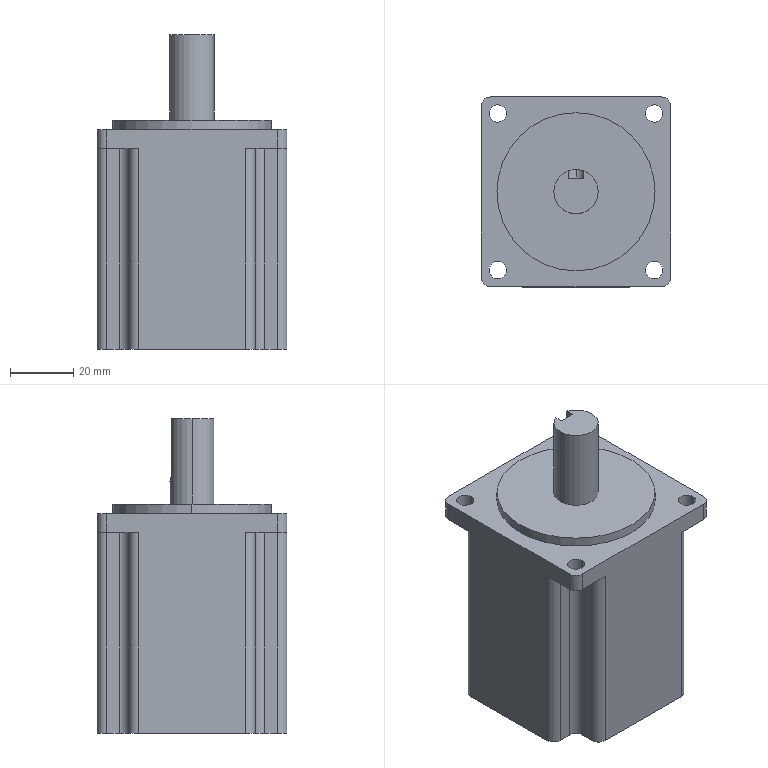Part | SolidWorks | features ICE 4, Fillet 3, Extrusion 1, HoleWzd 1 | 1 solid | 53 faces | box 60 x 60 x 99.5 mm | volume 233462 mm3 | cylinder 30 | plane 23 | commonest cylinder face diameters 6 x16 5.5 x8 5 x2 14 x2 50 x2